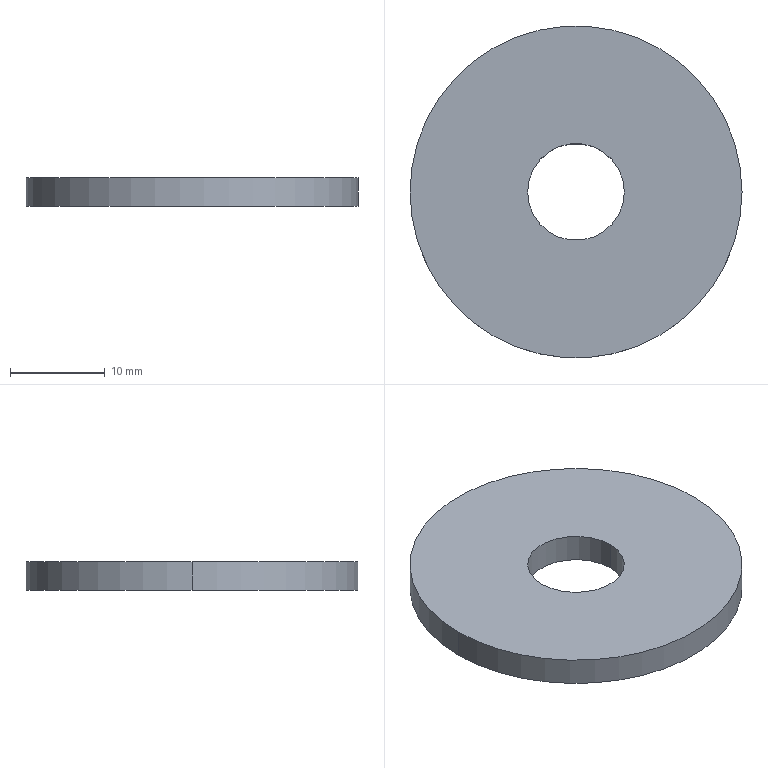Part | NX | features solid 2 | 1 solid | 6 faces | box 35 x 35 x 3 mm | volume 2641 mm3 | cylinder 4 | plane 2 | commonest cylinder face diameters 10.2 x2 35 x2
STEP:
#1=CARTESIAN_POINT('',(1184.9,-1523.,1290.));
#2=VERTEX_POINT('',#1);
#3=CARTESIAN_POINT('',(1184.9,-1523.,1293.));
#4=VERTEX_POINT('',#3);
#5=CARTESIAN_POINT('',(1184.9,-1523.,1339.588));
#6=DIRECTION('',(0.,0.,-1.));
#7=VECTOR('',#6,1000.);
#8=LINE('',#5,#7);
#9=EDGE_CURVE('',#2,#4,#8,.F.);
#10=ORIENTED_EDGE('',*,*,#9,.T.);
#11=CARTESIAN_POINT('',(1195.1,-1523.,1293.));
#12=VERTEX_POINT('',#11);
#13=CARTESIAN_POINT('',(1190.,-1523.,1293.));
#14=DIRECTION('',(0.,0.,1.));
#15=DIRECTION('',(-1.,0.,0.));
#16=AXIS2_PLACEMENT_3D('',#13,#14,#15);
#17=CIRCLE('',#16,5.1);
#18=EDGE_CURVE('',#4,#12,#17,.T.);
#19=ORIENTED_EDGE('',*,*,#18,.T.);
#20=CARTESIAN_POINT('',(1195.1,-1523.,1290.));
#21=VERTEX_POINT('',#20);
#22=CARTESIAN_POINT('',(1195.1,-1523.,1339.588));
#23=DIRECTION('',(0.,0.,-1.));
#24=VECTOR('',#23,1000.);
#25=LINE('',#22,#24);
#26=EDGE_CURVE('',#12,#21,#25,.T.);
#27=ORIENTED_EDGE('',*,*,#26,.T.);
#28=CARTESIAN_POINT('',(1190.,-1523.,1290.));
#29=DIRECTION('',(0.,0.,-1.));
#30=DIRECTION('',(1.,0.,0.));
#31=AXIS2_PLACEMENT_3D('',#28,#29,#30);
#32=CIRCLE('',#31,5.1);
#33=EDGE_CURVE('',#21,#2,#32,.T.);
#34=ORIENTED_EDGE('',*,*,#33,.T.);
#35=EDGE_LOOP('',(#10,#19,#27,#34));
#36=FACE_BOUND('',#35,.T.);
#37=CARTESIAN_POINT('',(1190.,-1523.,1339.588));
#38=DIRECTION('',(0.,0.,-1.));
#39=DIRECTION('',(1.,0.,0.));
#40=AXIS2_PLACEMENT_3D('',#37,#38,#39);
#41=CYLINDRICAL_SURFACE('',#40,5.1);
#42=ADVANCED_FACE('',(#36),#41,.F.);
#43=ORIENTED_EDGE('',*,*,#33,.F.);
#44=CARTESIAN_POINT('',(1190.,-1523.,1290.));
#45=DIRECTION('',(0.,0.,-1.));
#46=DIRECTION('',(1.,0.,0.));
#47=AXIS2_PLACEMENT_3D('',#44,#45,#46);
#48=CIRCLE('',#47,5.1);
#49=EDGE_CURVE('',#2,#21,#48,.T.);
#50=ORIENTED_EDGE('',*,*,#49,.F.);
#51=EDGE_LOOP('',(#43,#50));
#52=FACE_BOUND('',#51,.T.);
#53=CARTESIAN_POINT('',(1207.5,-1523.,1290.));
#54=VERTEX_POINT('',#53);
#55=CARTESIAN_POINT('',(1172.5,-1523.,1290.));
#56=VERTEX_POINT('',#55);
#57=CARTESIAN_POINT('',(1190.,-1523.,1290.));
#58=DIRECTION('',(0.,0.,1.));
#59=DIRECTION('',(1.,0.,0.));
#60=AXIS2_PLACEMENT_3D('',#57,#58,#59);
#61=CIRCLE('',#60,17.5);
#62=EDGE_CURVE('',#54,#56,#61,.T.);
#63=ORIENTED_EDGE('',*,*,#62,.F.);
#64=CARTESIAN_POINT('',(1190.,-1523.,1290.));
#65=DIRECTION('',(0.,0.,1.));
#66=DIRECTION('',(1.,0.,0.));
#67=AXIS2_PLACEMENT_3D('',#64,#65,#66);
#68=CIRCLE('',#67,17.5);
#69=EDGE_CURVE('',#56,#54,#68,.T.);
#70=ORIENTED_EDGE('',*,*,#69,.F.);
#71=EDGE_LOOP('',(#63,#70));
#72=FACE_BOUND('',#71,.T.);
#73=CARTESIAN_POINT('',(1190.,-1523.,1290.));
#74=DIRECTION('',(0.,0.,1.));
#75=DIRECTION('',(1.,0.,0.));
#76=AXIS2_PLACEMENT_3D('',#73,#74,#75);
#77=PLANE('',#76);
#78=ADVANCED_FACE('',(#52,#72),#77,.F.);
#79=CARTESIAN_POINT('',(1190.,-1523.,1293.));
#80=DIRECTION('',(0.,0.,1.));
#81=DIRECTION('',(-1.,0.,0.));
#82=AXIS2_PLACEMENT_3D('',#79,#80,#81);
#83=CIRCLE('',#82,5.1);
#84=EDGE_CURVE('',#12,#4,#83,.T.);
#85=ORIENTED_EDGE('',*,*,#84,.F.);
#86=ORIENTED_EDGE('',*,*,#18,.F.);
#87=EDGE_LOOP('',(#85,#86));
#88=FACE_BOUND('',#87,.T.);
#89=CARTESIAN_POINT('',(1207.5,-1523.,1293.));
#90=VERTEX_POINT('',#89);
#91=CARTESIAN_POINT('',(1172.5,-1523.,1293.));
#92=VERTEX_POINT('',#91);
#93=CARTESIAN_POINT('',(1190.,-1523.,1293.));
#94=DIRECTION('',(0.,0.,1.));
#95=DIRECTION('',(1.,0.,0.));
#96=AXIS2_PLACEMENT_3D('',#93,#94,#95);
#97=CIRCLE('',#96,17.5);
#98=EDGE_CURVE('',#90,#92,#97,.T.);
#99=ORIENTED_EDGE('',*,*,#98,.T.);
#100=CARTESIAN_POINT('',(1190.,-1523.,1293.));
#101=DIRECTION('',(0.,0.,1.));
#102=DIRECTION('',(1.,0.,0.));
#103=AXIS2_PLACEMENT_3D('',#100,#101,#102);
#104=CIRCLE('',#103,17.5);
#105=EDGE_CURVE('',#92,#90,#104,.T.);
#106=ORIENTED_EDGE('',*,*,#105,.T.);
#107=EDGE_LOOP('',(#99,#106));
#108=FACE_BOUND('',#107,.T.);
#109=CARTESIAN_POINT('',(1190.,-1523.,1293.));
#110=DIRECTION('',(0.,0.,1.));
#111=DIRECTION('',(1.,0.,0.));
#112=AXIS2_PLACEMENT_3D('',#109,#110,#111);
#113=PLANE('',#112);
#114=ADVANCED_FACE('',(#88,#108),#113,.T.);
#115=CARTESIAN_POINT('',(1172.5,-1523.,1293.));
#116=DIRECTION('',(0.,0.,-1.));
#117=VECTOR('',#116,1000.);
#118=LINE('',#115,#117);
#119=EDGE_CURVE('',#56,#92,#118,.F.);
#120=ORIENTED_EDGE('',*,*,#119,.T.);
#121=ORIENTED_EDGE('',*,*,#98,.F.);
#122=CARTESIAN_POINT('',(1207.5,-1523.,1293.));
#123=DIRECTION('',(0.,0.,-1.));
#124=VECTOR('',#123,1000.);
#125=LINE('',#122,#124);
#126=EDGE_CURVE('',#90,#54,#125,.T.);
#127=ORIENTED_EDGE('',*,*,#126,.T.);
#128=ORIENTED_EDGE('',*,*,#62,.T.);
#129=EDGE_LOOP('',(#120,#121,#127,#128));
#130=FACE_BOUND('',#129,.T.);
#131=CARTESIAN_POINT('',(1190.,-1523.,1293.));
#132=DIRECTION('',(0.,0.,-1.));
#133=DIRECTION('',(1.,0.,0.));
#134=AXIS2_PLACEMENT_3D('',#131,#132,#133);
#135=CYLINDRICAL_SURFACE('',#134,17.5);
#136=ADVANCED_FACE('',(#130),#135,.T.);
#137=ORIENTED_EDGE('',*,*,#105,.F.);
#138=ORIENTED_EDGE('',*,*,#119,.F.);
#139=ORIENTED_EDGE('',*,*,#69,.T.);
#140=ORIENTED_EDGE('',*,*,#126,.F.);
#141=EDGE_LOOP('',(#137,#138,#139,#140));
#142=FACE_BOUND('',#141,.T.);
#143=CARTESIAN_POINT('',(1190.,-1523.,1293.));
#144=DIRECTION('',(0.,0.,-1.));
#145=DIRECTION('',(1.,0.,0.));
#146=AXIS2_PLACEMENT_3D('',#143,#144,#145);
#147=CYLINDRICAL_SURFACE('',#146,17.5);
#148=ADVANCED_FACE('',(#142),#147,.T.);
#149=ORIENTED_EDGE('',*,*,#84,.T.);
#150=ORIENTED_EDGE('',*,*,#9,.F.);
#151=ORIENTED_EDGE('',*,*,#49,.T.);
#152=ORIENTED_EDGE('',*,*,#26,.F.);
#153=EDGE_LOOP('',(#149,#150,#151,#152));
#154=FACE_BOUND('',#153,.T.);
#155=CARTESIAN_POINT('',(1190.,-1523.,1339.588));
#156=DIRECTION('',(0.,0.,-1.));
#157=DIRECTION('',(1.,0.,0.));
#158=AXIS2_PLACEMENT_3D('',#155,#156,#157);
#159=CYLINDRICAL_SURFACE('',#158,5.1);
#160=ADVANCED_FACE('',(#154),#159,.F.);
#161=CLOSED_SHELL('',(#42,#78,#114,#136,#148,#160));
#162=MANIFOLD_SOLID_BREP('',#161);
#163=(LENGTH_UNIT()NAMED_UNIT(*)SI_UNIT(.MILLI.,.METRE.));
#164=UNCERTAINTY_MEASURE_WITH_UNIT(LENGTH_MEASURE(0.00001),#163,'','');
#165=(NAMED_UNIT(*)PLANE_ANGLE_UNIT()SI_UNIT($,.RADIAN.));
#166=(NAMED_UNIT(*)SI_UNIT($,.STERADIAN.)SOLID_ANGLE_UNIT());
#167=(GEOMETRIC_REPRESENTATION_CONTEXT(3)GLOBAL_UNCERTAINTY_ASSIGNED_CONTEXT((#164))GLOBAL_UNIT_ASSIGNED_CONTEXT((#163,#165,#166))REPRESENTATION_CONTEXT('',''));
#168=ADVANCED_BREP_SHAPE_REPRESENTATION('',(#162),#167);